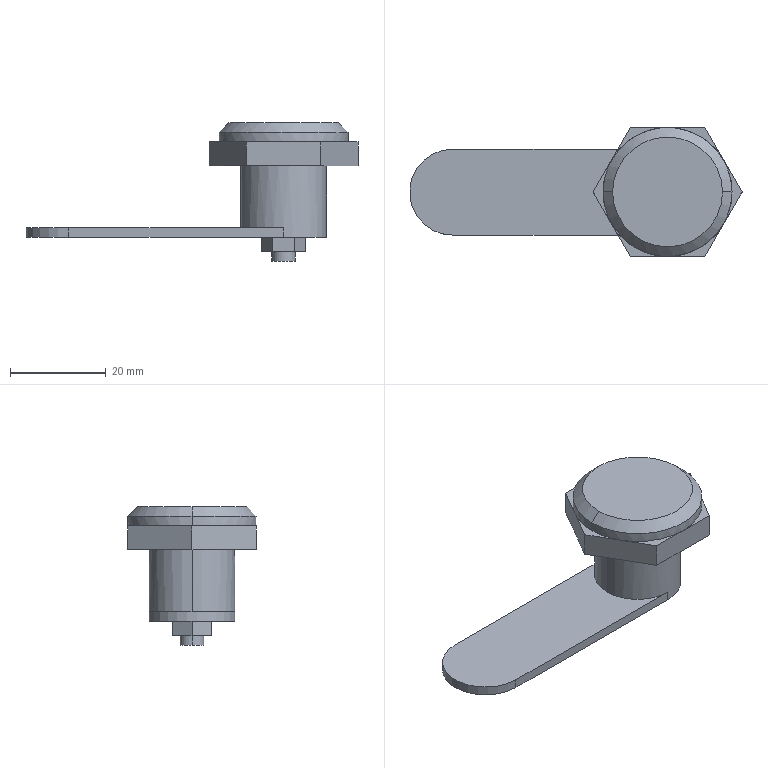Part | SolidWorks | features ICE 5, Chamfer 1, Extrusion 1 | 1 solid | 35 faces | box 69.588 x 27 x 29 mm | volume 10928 mm3 | plane 26 | cylinder 7 | cone 2 | commonest cylinder face diameters 18 x3 5 x2 27 x2
STEP:
#1=CARTESIAN_POINT('',(-2.5,0.,-25.));
#2=VERTEX_POINT('',#1);
#3=CARTESIAN_POINT('',(2.5,0.,-25.));
#4=VERTEX_POINT('',#3);
#5=CARTESIAN_POINT('',(0.,0.,-25.));
#6=DIRECTION('',(0.,0.,-1.));
#7=DIRECTION('',(-1.,0.,0.));
#8=AXIS2_PLACEMENT_3D('',#5,#6,#7);
#9=CIRCLE('',#8,2.5);
#10=EDGE_CURVE('',#2,#4,#9,.T.);
#11=ORIENTED_EDGE('',*,*,#10,.F.);
#12=CARTESIAN_POINT('',(-2.5,0.,-23.));
#13=VERTEX_POINT('',#12);
#14=CARTESIAN_POINT('',(-2.5,0.,-25.));
#15=DIRECTION('',(0.,0.,1.));
#16=VECTOR('',#15,1000.);
#17=LINE('',#14,#16);
#18=EDGE_CURVE('',#2,#13,#17,.T.);
#19=ORIENTED_EDGE('',*,*,#18,.T.);
#20=CARTESIAN_POINT('',(2.5,0.,-23.));
#21=VERTEX_POINT('',#20);
#22=CARTESIAN_POINT('',(0.,0.,-23.));
#23=DIRECTION('',(0.,0.,-1.));
#24=DIRECTION('',(-1.,0.,0.));
#25=AXIS2_PLACEMENT_3D('',#22,#23,#24);
#26=CIRCLE('',#25,2.5);
#27=EDGE_CURVE('',#13,#21,#26,.T.);
#28=ORIENTED_EDGE('',*,*,#27,.T.);
#29=CARTESIAN_POINT('',(2.5,0.,-25.));
#30=DIRECTION('',(0.,0.,1.));
#31=VECTOR('',#30,1000.);
#32=LINE('',#29,#31);
#33=EDGE_CURVE('',#4,#21,#32,.T.);
#34=ORIENTED_EDGE('',*,*,#33,.F.);
#35=EDGE_LOOP('',(#11,#19,#28,#34));
#36=FACE_OUTER_BOUND('',#35,.T.);
#37=CARTESIAN_POINT('',(0.,0.,-25.));
#38=DIRECTION('',(0.,0.,1.));
#39=DIRECTION('',(1.,0.,0.));
#40=AXIS2_PLACEMENT_3D('',#37,#38,#39);
#41=CYLINDRICAL_SURFACE('',#40,2.5);
#42=ADVANCED_FACE('',(#36),#41,.T.);
#43=CARTESIAN_POINT('',(-9.,0.,-18.));
#44=VERTEX_POINT('',#43);
#45=CARTESIAN_POINT('',(0.,9.,-18.));
#46=VERTEX_POINT('',#45);
#47=CARTESIAN_POINT('',(0.,0.,-18.));
#48=DIRECTION('',(0.,0.,-1.));
#49=DIRECTION('',(-1.,0.,0.));
#50=AXIS2_PLACEMENT_3D('',#47,#48,#49);
#51=CIRCLE('',#50,9.);
#52=EDGE_CURVE('',#44,#46,#51,.T.);
#53=ORIENTED_EDGE('',*,*,#52,.F.);
#54=CARTESIAN_POINT('',(-9.,0.,-5.));
#55=VERTEX_POINT('',#54);
#56=CARTESIAN_POINT('',(-9.,0.,-18.));
#57=DIRECTION('',(0.,0.,1.));
#58=VECTOR('',#57,1000.);
#59=LINE('',#56,#58);
#60=EDGE_CURVE('',#44,#55,#59,.T.);
#61=ORIENTED_EDGE('',*,*,#60,.T.);
#62=CARTESIAN_POINT('',(9.,0.,-5.));
#63=VERTEX_POINT('',#62);
#64=CARTESIAN_POINT('',(0.,0.,-5.));
#65=DIRECTION('',(0.,0.,-1.));
#66=DIRECTION('',(-1.,0.,0.));
#67=AXIS2_PLACEMENT_3D('',#64,#65,#66);
#68=CIRCLE('',#67,9.);
#69=EDGE_CURVE('',#55,#63,#68,.T.);
#70=ORIENTED_EDGE('',*,*,#69,.T.);
#71=CARTESIAN_POINT('',(9.,0.,-20.));
#72=VERTEX_POINT('',#71);
#73=CARTESIAN_POINT('',(9.,0.,-18.));
#74=DIRECTION('',(0.,0.,1.));
#75=VECTOR('',#74,1000.);
#76=LINE('',#73,#75);
#77=EDGE_CURVE('',#72,#63,#76,.T.);
#78=ORIENTED_EDGE('',*,*,#77,.F.);
#79=CARTESIAN_POINT('',(0.,9.,-20.));
#80=VERTEX_POINT('',#79);
#81=CARTESIAN_POINT('',(0.,0.,-20.));
#82=DIRECTION('',(0.,0.,-1.));
#83=DIRECTION('',(-1.,0.,0.));
#84=AXIS2_PLACEMENT_3D('',#81,#82,#83);
#85=CIRCLE('',#84,9.);
#86=EDGE_CURVE('',#80,#72,#85,.T.);
#87=ORIENTED_EDGE('',*,*,#86,.F.);
#88=CARTESIAN_POINT('',(0.,9.,-20.));
#89=DIRECTION('',(0.,0.,1.));
#90=VECTOR('',#89,1000.);
#91=LINE('',#88,#90);
#92=EDGE_CURVE('',#80,#46,#91,.T.);
#93=ORIENTED_EDGE('',*,*,#92,.T.);
#94=EDGE_LOOP('',(#53,#61,#70,#78,#87,#93));
#95=FACE_OUTER_BOUND('',#94,.T.);
#96=CARTESIAN_POINT('',(0.,0.,-18.));
#97=DIRECTION('',(0.,0.,1.));
#98=DIRECTION('',(1.,0.,0.));
#99=AXIS2_PLACEMENT_3D('',#96,#97,#98);
#100=CYLINDRICAL_SURFACE('',#99,9.);
#101=ADVANCED_FACE('',(#95),#100,.T.);
#102=CARTESIAN_POINT('',(11.5,0.,4.));
#103=VERTEX_POINT('',#102);
#104=CARTESIAN_POINT('',(-11.5,0.,4.));
#105=VERTEX_POINT('',#104);
#106=CARTESIAN_POINT('',(0.,0.,4.));
#107=DIRECTION('',(0.,0.,1.));
#108=DIRECTION('',(1.,0.,0.));
#109=AXIS2_PLACEMENT_3D('',#106,#107,#108);
#110=CIRCLE('',#109,11.5);
#111=EDGE_CURVE('',#103,#105,#110,.T.);
#112=ORIENTED_EDGE('',*,*,#111,.F.);
#113=CARTESIAN_POINT('',(13.5,0.,2.));
#114=VERTEX_POINT('',#113);
#115=CARTESIAN_POINT('',(11.5,0.,4.));
#116=DIRECTION('',(0.7071,0.,-0.7071));
#117=VECTOR('',#116,1000.);
#118=LINE('',#115,#117);
#119=EDGE_CURVE('',#103,#114,#118,.T.);
#120=ORIENTED_EDGE('',*,*,#119,.T.);
#121=CARTESIAN_POINT('',(-13.5,0.,2.));
#122=VERTEX_POINT('',#121);
#123=CARTESIAN_POINT('',(0.,0.,2.));
#124=DIRECTION('',(0.,0.,-1.));
#125=DIRECTION('',(1.,0.,0.));
#126=AXIS2_PLACEMENT_3D('',#123,#124,#125);
#127=CIRCLE('',#126,13.5);
#128=EDGE_CURVE('',#122,#114,#127,.T.);
#129=ORIENTED_EDGE('',*,*,#128,.F.);
#130=CARTESIAN_POINT('',(-11.5,0.,4.));
#131=DIRECTION('',(-0.7071,0.,-0.7071));
#132=VECTOR('',#131,1000.);
#133=LINE('',#130,#132);
#134=EDGE_CURVE('',#105,#122,#133,.T.);
#135=ORIENTED_EDGE('',*,*,#134,.F.);
#136=EDGE_LOOP('',(#112,#120,#129,#135));
#137=FACE_OUTER_BOUND('',#136,.T.);
#138=CARTESIAN_POINT('',(0.,0.,4.));
#139=DIRECTION('',(0.,0.,-1.));
#140=DIRECTION('',(-1.,0.,0.));
#141=AXIS2_PLACEMENT_3D('',#138,#139,#140);
#142=CONICAL_SURFACE('',#141,11.5,0.7854);
#143=ADVANCED_FACE('',(#137),#142,.T.);
#144=ORIENTED_EDGE('',*,*,#128,.T.);
#145=CARTESIAN_POINT('',(13.5,0.,0.));
#146=VERTEX_POINT('',#145);
#147=CARTESIAN_POINT('',(13.5,0.,4.));
#148=DIRECTION('',(0.,0.,-1.));
#149=VECTOR('',#148,1000.);
#150=LINE('',#147,#149);
#151=EDGE_CURVE('',#114,#146,#150,.T.);
#152=ORIENTED_EDGE('',*,*,#151,.T.);
#153=CARTESIAN_POINT('',(11.691,6.75,0.));
#154=VERTEX_POINT('',#153);
#155=CARTESIAN_POINT('',(0.,0.,0.));
#156=DIRECTION('',(0.,0.,1.));
#157=DIRECTION('',(1.,0.,0.));
#158=AXIS2_PLACEMENT_3D('',#155,#156,#157);
#159=CIRCLE('',#158,13.5);
#160=EDGE_CURVE('',#146,#154,#159,.T.);
#161=ORIENTED_EDGE('',*,*,#160,.T.);
#162=CARTESIAN_POINT('',(0.,13.5,0.));
#163=VERTEX_POINT('',#162);
#164=CARTESIAN_POINT('',(0.,0.,0.));
#165=DIRECTION('',(0.,0.,1.));
#166=DIRECTION('',(1.,0.,0.));
#167=AXIS2_PLACEMENT_3D('',#164,#165,#166);
#168=CIRCLE('',#167,13.5);
#169=EDGE_CURVE('',#154,#163,#168,.T.);
#170=ORIENTED_EDGE('',*,*,#169,.T.);
#171=CARTESIAN_POINT('',(-11.691,6.75,0.));
#172=VERTEX_POINT('',#171);
#173=CARTESIAN_POINT('',(0.,0.,0.));
#174=DIRECTION('',(0.,0.,1.));
#175=DIRECTION('',(1.,0.,0.));
#176=AXIS2_PLACEMENT_3D('',#173,#174,#175);
#177=CIRCLE('',#176,13.5);
#178=EDGE_CURVE('',#163,#172,#177,.T.);
#179=ORIENTED_EDGE('',*,*,#178,.T.);
#180=CARTESIAN_POINT('',(-13.5,0.,0.));
#181=VERTEX_POINT('',#180);
#182=CARTESIAN_POINT('',(0.,0.,0.));
#183=DIRECTION('',(0.,0.,1.));
#184=DIRECTION('',(1.,0.,0.));
#185=AXIS2_PLACEMENT_3D('',#182,#183,#184);
#186=CIRCLE('',#185,13.5);
#187=EDGE_CURVE('',#172,#181,#186,.T.);
#188=ORIENTED_EDGE('',*,*,#187,.T.);
#189=CARTESIAN_POINT('',(-13.5,0.,4.));
#190=DIRECTION('',(0.,0.,-1.));
#191=VECTOR('',#190,1000.);
#192=LINE('',#189,#191);
#193=EDGE_CURVE('',#122,#181,#192,.T.);
#194=ORIENTED_EDGE('',*,*,#193,.F.);
#195=EDGE_LOOP('',(#144,#152,#161,#170,#179,#188,#194));
#196=FACE_OUTER_BOUND('',#195,.T.);
#197=CARTESIAN_POINT('',(0.,0.,4.));
#198=DIRECTION('',(0.,0.,-1.));
#199=DIRECTION('',(-1.,0.,0.));
#200=AXIS2_PLACEMENT_3D('',#197,#198,#199);
#201=CYLINDRICAL_SURFACE('',#200,13.5);
#202=ADVANCED_FACE('',(#196),#201,.T.);
#203=ORIENTED_EDGE('',*,*,#86,.T.);
#204=CARTESIAN_POINT('',(0.,-9.,-20.));
#205=VERTEX_POINT('',#204);
#206=CARTESIAN_POINT('',(0.,0.,-20.));
#207=DIRECTION('',(0.,0.,-1.));
#208=DIRECTION('',(-1.,0.,0.));
#209=AXIS2_PLACEMENT_3D('',#206,#207,#208);
#210=CIRCLE('',#209,9.);
#211=EDGE_CURVE('',#72,#205,#210,.T.);
#212=ORIENTED_EDGE('',*,*,#211,.T.);
#213=CARTESIAN_POINT('',(-45.,-9.,-20.));
#214=VERTEX_POINT('',#213);
#215=CARTESIAN_POINT('',(0.,-9.,-20.));
#216=DIRECTION('',(-1.,0.,0.));
#217=VECTOR('',#216,1000.);
#218=LINE('',#215,#217);
#219=EDGE_CURVE('',#205,#214,#218,.T.);
#220=ORIENTED_EDGE('',*,*,#219,.T.);
#221=CARTESIAN_POINT('',(-45.,9.,-20.));
#222=VERTEX_POINT('',#221);
#223=CARTESIAN_POINT('',(-45.,0.,-20.));
#224=DIRECTION('',(0.,0.,-1.));
#225=DIRECTION('',(-1.,0.,0.));
#226=AXIS2_PLACEMENT_3D('',#223,#224,#225);
#227=CIRCLE('',#226,9.);
#228=EDGE_CURVE('',#214,#222,#227,.T.);
#229=ORIENTED_EDGE('',*,*,#228,.T.);
#230=CARTESIAN_POINT('',(0.,9.,-20.));
#231=DIRECTION('',(1.,0.,0.));
#232=VECTOR('',#231,1000.);
#233=LINE('',#230,#232);
#234=EDGE_CURVE('',#222,#80,#233,.T.);
#235=ORIENTED_EDGE('',*,*,#234,.T.);
#236=EDGE_LOOP('',(#203,#212,#220,#229,#235));
#237=FACE_OUTER_BOUND('',#236,.T.);
#238=CARTESIAN_POINT('',(2.309,-4.,-20.));
#239=VERTEX_POINT('',#238);
#240=CARTESIAN_POINT('',(-2.309,-4.,-20.));
#241=VERTEX_POINT('',#240);
#242=CARTESIAN_POINT('',(2.309,-4.,-20.));
#243=DIRECTION('',(-1.,0.,0.));
#244=VECTOR('',#243,1000.);
#245=LINE('',#242,#244);
#246=EDGE_CURVE('',#239,#241,#245,.T.);
#247=ORIENTED_EDGE('',*,*,#246,.F.);
#248=CARTESIAN_POINT('',(4.619,0.,-20.));
#249=VERTEX_POINT('',#248);
#250=CARTESIAN_POINT('',(4.619,0.,-20.));
#251=DIRECTION('',(-0.5,-0.866,0.));
#252=VECTOR('',#251,1000.);
#253=LINE('',#250,#252);
#254=EDGE_CURVE('',#249,#239,#253,.T.);
#255=ORIENTED_EDGE('',*,*,#254,.F.);
#256=CARTESIAN_POINT('',(2.309,4.,-20.));
#257=VERTEX_POINT('',#256);
#258=CARTESIAN_POINT('',(2.309,4.,-20.));
#259=DIRECTION('',(0.5,-0.866,0.));
#260=VECTOR('',#259,1000.);
#261=LINE('',#258,#260);
#262=EDGE_CURVE('',#257,#249,#261,.T.);
#263=ORIENTED_EDGE('',*,*,#262,.F.);
#264=CARTESIAN_POINT('',(-2.309,4.,-20.));
#265=VERTEX_POINT('',#264);
#266=CARTESIAN_POINT('',(-2.309,4.,-20.));
#267=DIRECTION('',(1.,0.,0.));
#268=VECTOR('',#267,1000.);
#269=LINE('',#266,#268);
#270=EDGE_CURVE('',#265,#257,#269,.T.);
#271=ORIENTED_EDGE('',*,*,#270,.F.);
#272=CARTESIAN_POINT('',(-4.619,0.,-20.));
#273=VERTEX_POINT('',#272);
#274=CARTESIAN_POINT('',(-4.619,0.,-20.));
#275=DIRECTION('',(0.5,0.866,0.));
#276=VECTOR('',#275,1000.);
#277=LINE('',#274,#276);
#278=EDGE_CURVE('',#273,#265,#277,.T.);
#279=ORIENTED_EDGE('',*,*,#278,.F.);
#280=CARTESIAN_POINT('',(-2.309,-4.,-20.));
#281=DIRECTION('',(-0.5,0.866,0.));
#282=VECTOR('',#281,1000.);
#283=LINE('',#280,#282);
#284=EDGE_CURVE('',#241,#273,#283,.T.);
#285=ORIENTED_EDGE('',*,*,#284,.F.);
#286=EDGE_LOOP('',(#247,#255,#263,#271,#279,#285));
#287=FACE_BOUND('',#286,.T.);
#288=CARTESIAN_POINT('',(0.,0.,-20.));
#289=DIRECTION('',(0.,0.,-1.));
#290=DIRECTION('',(-1.,0.,0.));
#291=AXIS2_PLACEMENT_3D('',#288,#289,#290);
#292=PLANE('',#291);
#293=ADVANCED_FACE('',(#237,#287),#292,.T.);
#294=CARTESIAN_POINT('',(7.794,13.5,-5.));
#295=VERTEX_POINT('',#294);
#296=CARTESIAN_POINT('',(15.588,0.,-5.));
#297=VERTEX_POINT('',#296);
#298=CARTESIAN_POINT('',(7.794,13.5,-5.));
#299=DIRECTION('',(0.5,-0.866,0.));
#300=VECTOR('',#299,1000.);
#301=LINE('',#298,#300);
#302=EDGE_CURVE('',#295,#297,#301,.T.);
#303=ORIENTED_EDGE('',*,*,#302,.T.);
#304=CARTESIAN_POINT('',(7.794,-13.5,-5.));
#305=VERTEX_POINT('',#304);
#306=CARTESIAN_POINT('',(15.588,0.,-5.));
#307=DIRECTION('',(-0.5,-0.866,0.));
#308=VECTOR('',#307,1000.);
#309=LINE('',#306,#308);
#310=EDGE_CURVE('',#297,#305,#309,.T.);
#311=ORIENTED_EDGE('',*,*,#310,.T.);
#312=CARTESIAN_POINT('',(-7.794,-13.5,-5.));
#313=VERTEX_POINT('',#312);
#314=CARTESIAN_POINT('',(7.794,-13.5,-5.));
#315=DIRECTION('',(-1.,0.,0.));
#316=VECTOR('',#315,1000.);
#317=LINE('',#314,#316);
#318=EDGE_CURVE('',#305,#313,#317,.T.);
#319=ORIENTED_EDGE('',*,*,#318,.T.);
#320=CARTESIAN_POINT('',(-15.588,0.,-5.));
#321=VERTEX_POINT('',#320);
#322=CARTESIAN_POINT('',(-7.794,-13.5,-5.));
#323=DIRECTION('',(-0.5,0.866,0.));
#324=VECTOR('',#323,1000.);
#325=LINE('',#322,#324);
#326=EDGE_CURVE('',#313,#321,#325,.T.);
#327=ORIENTED_EDGE('',*,*,#326,.T.);
#328=CARTESIAN_POINT('',(-7.794,13.5,-5.));
#329=VERTEX_POINT('',#328);
#330=CARTESIAN_POINT('',(-15.588,0.,-5.));
#331=DIRECTION('',(0.5,0.866,0.));
#332=VECTOR('',#331,1000.);
#333=LINE('',#330,#332);
#334=EDGE_CURVE('',#321,#329,#333,.T.);
#335=ORIENTED_EDGE('',*,*,#334,.T.);
#336=CARTESIAN_POINT('',(-7.794,13.5,-5.));
#337=DIRECTION('',(1.,0.,0.));
#338=VECTOR('',#337,1000.);
#339=LINE('',#336,#338);
#340=EDGE_CURVE('',#329,#295,#339,.T.);
#341=ORIENTED_EDGE('',*,*,#340,.T.);
#342=EDGE_LOOP('',(#303,#311,#319,#327,#335,#341));
#343=FACE_OUTER_BOUND('',#342,.T.);
#344=CARTESIAN_POINT('',(0.,0.,-5.));
#345=DIRECTION('',(0.,0.,-1.));
#346=DIRECTION('',(-1.,0.,0.));
#347=AXIS2_PLACEMENT_3D('',#344,#345,#346);
#348=CIRCLE('',#347,9.);
#349=EDGE_CURVE('',#63,#55,#348,.T.);
#350=ORIENTED_EDGE('',*,*,#349,.F.);
#351=ORIENTED_EDGE('',*,*,#69,.F.);
#352=EDGE_LOOP('',(#350,#351));
#353=FACE_BOUND('',#352,.T.);
#354=CARTESIAN_POINT('',(15.588,0.,-5.));
#355=DIRECTION('',(0.,0.,-1.));
#356=DIRECTION('',(-1.,0.,0.));
#357=AXIS2_PLACEMENT_3D('',#354,#355,#356);
#358=PLANE('',#357);
#359=ADVANCED_FACE('',(#343,#353),#358,.T.);
#360=ORIENTED_EDGE('',*,*,#151,.F.);
#361=CARTESIAN_POINT('',(0.,0.,2.));
#362=DIRECTION('',(0.,0.,-1.));
#363=DIRECTION('',(1.,0.,0.));
#364=AXIS2_PLACEMENT_3D('',#361,#362,#363);
#365=CIRCLE('',#364,13.5);
#366=EDGE_CURVE('',#114,#122,#365,.T.);
#367=ORIENTED_EDGE('',*,*,#366,.T.);
#368=ORIENTED_EDGE('',*,*,#193,.T.);
#369=CARTESIAN_POINT('',(-11.691,-6.75,0.));
#370=VERTEX_POINT('',#369);
#371=CARTESIAN_POINT('',(0.,0.,0.));
#372=DIRECTION('',(0.,0.,1.));
#373=DIRECTION('',(1.,0.,0.));
#374=AXIS2_PLACEMENT_3D('',#371,#372,#373);
#375=CIRCLE('',#374,13.5);
#376=EDGE_CURVE('',#181,#370,#375,.T.);
#377=ORIENTED_EDGE('',*,*,#376,.T.);
#378=CARTESIAN_POINT('',(0.,-13.5,0.));
#379=VERTEX_POINT('',#378);
#380=CARTESIAN_POINT('',(0.,0.,0.));
#381=DIRECTION('',(0.,0.,1.));
#382=DIRECTION('',(1.,0.,0.));
#383=AXIS2_PLACEMENT_3D('',#380,#381,#382);
#384=CIRCLE('',#383,13.5);
#385=EDGE_CURVE('',#370,#379,#384,.T.);
#386=ORIENTED_EDGE('',*,*,#385,.T.);
#387=CARTESIAN_POINT('',(11.691,-6.75,0.));
#388=VERTEX_POINT('',#387);
#389=CARTESIAN_POINT('',(0.,0.,0.));
#390=DIRECTION('',(0.,0.,1.));
#391=DIRECTION('',(1.,0.,0.));
#392=AXIS2_PLACEMENT_3D('',#389,#390,#391);
#393=CIRCLE('',#392,13.5);
#394=EDGE_CURVE('',#379,#388,#393,.T.);
#395=ORIENTED_EDGE('',*,*,#394,.T.);
#396=CARTESIAN_POINT('',(0.,0.,0.));
#397=DIRECTION('',(0.,0.,1.));
#398=DIRECTION('',(1.,0.,0.));
#399=AXIS2_PLACEMENT_3D('',#396,#397,#398);
#400=CIRCLE('',#399,13.5);
#401=EDGE_CURVE('',#388,#146,#400,.T.);
#402=ORIENTED_EDGE('',*,*,#401,.T.);
#403=EDGE_LOOP('',(#360,#367,#368,#377,#386,#395,#402));
#404=FACE_OUTER_BOUND('',#403,.T.);
#405=CARTESIAN_POINT('',(0.,0.,4.));
#406=DIRECTION('',(0.,0.,-1.));
#407=DIRECTION('',(-1.,0.,0.));
#408=AXIS2_PLACEMENT_3D('',#405,#406,#407);
#409=CYLINDRICAL_SURFACE('',#408,13.5);
#410=ADVANCED_FACE('',(#404),#409,.T.);
#411=CARTESIAN_POINT('',(0.,0.,4.));
#412=DIRECTION('',(0.,0.,1.));
#413=DIRECTION('',(1.,0.,0.));
#414=AXIS2_PLACEMENT_3D('',#411,#412,#413);
#415=CIRCLE('',#414,11.5);
#416=EDGE_CURVE('',#105,#103,#415,.T.);
#417=ORIENTED_EDGE('',*,*,#416,.T.);
#418=ORIENTED_EDGE('',*,*,#111,.T.);
#419=EDGE_LOOP('',(#417,#418));
#420=FACE_OUTER_BOUND('',#419,.T.);
#421=CARTESIAN_POINT('',(0.,0.,4.));
#422=DIRECTION('',(0.,0.,1.));
#423=DIRECTION('',(1.,0.,0.));
#424=AXIS2_PLACEMENT_3D('',#421,#422,#423);
#425=PLANE('',#424);
#426=ADVANCED_FACE('',(#420),#425,.T.);
#427=ORIENTED_EDGE('',*,*,#119,.F.);
#428=ORIENTED_EDGE('',*,*,#416,.F.);
#429=ORIENTED_EDGE('',*,*,#134,.T.);
#430=ORIENTED_EDGE('',*,*,#366,.F.);
#431=EDGE_LOOP('',(#427,#428,#429,#430));
#432=FACE_OUTER_BOUND('',#431,.T.);
#433=CARTESIAN_POINT('',(0.,0.,4.));
#434=DIRECTION('',(0.,0.,-1.));
#435=DIRECTION('',(-1.,0.,0.));
#436=AXIS2_PLACEMENT_3D('',#433,#434,#435);
#437=CONICAL_SURFACE('',#436,11.5,0.7854);
#438=ADVANCED_FACE('',(#432),#437,.T.);
#439=ORIENTED_EDGE('',*,*,#169,.F.);
#440=CARTESIAN_POINT('',(7.794,13.5,0.));
#441=VERTEX_POINT('',#440);
#442=CARTESIAN_POINT('',(7.794,13.5,0.));
#443=DIRECTION('',(0.5,-0.866,0.));
#444=VECTOR('',#443,1000.);
#445=LINE('',#442,#444);
#446=EDGE_CURVE('',#441,#154,#445,.T.);
#447=ORIENTED_EDGE('',*,*,#446,.F.);
#448=CARTESIAN_POINT('',(-7.794,13.5,0.));
#449=DIRECTION('',(1.,0.,0.));
#450=VECTOR('',#449,1000.);
#451=LINE('',#448,#450);
#452=EDGE_CURVE('',#163,#441,#451,.T.);
#453=ORIENTED_EDGE('',*,*,#452,.F.);
#454=EDGE_LOOP('',(#439,#447,#453));
#455=FACE_OUTER_BOUND('',#454,.T.);
#456=CARTESIAN_POINT('',(15.588,0.,0.));
#457=DIRECTION('',(0.,0.,-1.));
#458=DIRECTION('',(-1.,0.,0.));
#459=AXIS2_PLACEMENT_3D('',#456,#457,#458);
#460=PLANE('',#459);
#461=ADVANCED_FACE('',(#455),#460,.F.);
#462=ORIENTED_EDGE('',*,*,#178,.F.);
#463=CARTESIAN_POINT('',(-7.794,13.5,0.));
#464=VERTEX_POINT('',#463);
#465=CARTESIAN_POINT('',(-7.794,13.5,0.));
#466=DIRECTION('',(1.,0.,0.));
#467=VECTOR('',#466,1000.);
#468=LINE('',#465,#467);
#469=EDGE_CURVE('',#464,#163,#468,.T.);
#470=ORIENTED_EDGE('',*,*,#469,.F.);
#471=CARTESIAN_POINT('',(-15.588,0.,0.));
#472=DIRECTION('',(0.5,0.866,0.));
#473=VECTOR('',#472,1000.);
#474=LINE('',#471,#473);
#475=EDGE_CURVE('',#172,#464,#474,.T.);
#476=ORIENTED_EDGE('',*,*,#475,.F.);
#477=EDGE_LOOP('',(#462,#470,#476));
#478=FACE_OUTER_BOUND('',#477,.T.);
#479=CARTESIAN_POINT('',(15.588,0.,0.));
#480=DIRECTION('',(0.,0.,-1.));
#481=DIRECTION('',(-1.,0.,0.));
#482=AXIS2_PLACEMENT_3D('',#479,#480,#481);
#483=PLANE('',#482);
#484=ADVANCED_FACE('',(#478),#483,.F.);
#485=ORIENTED_EDGE('',*,*,#187,.F.);
#486=CARTESIAN_POINT('',(-15.588,0.,0.));
#487=VERTEX_POINT('',#486);
#488=CARTESIAN_POINT('',(-15.588,0.,0.));
#489=DIRECTION('',(0.5,0.866,0.));
#490=VECTOR('',#489,1000.);
#491=LINE('',#488,#490);
#492=EDGE_CURVE('',#487,#172,#491,.T.);
#493=ORIENTED_EDGE('',*,*,#492,.F.);
#494=CARTESIAN_POINT('',(-7.794,-13.5,0.));
#495=DIRECTION('',(-0.5,0.866,0.));
#496=VECTOR('',#495,1000.);
#497=LINE('',#494,#496);
#498=EDGE_CURVE('',#370,#487,#497,.T.);
#499=ORIENTED_EDGE('',*,*,#498,.F.);
#500=ORIENTED_EDGE('',*,*,#376,.F.);
#501=EDGE_LOOP('',(#485,#493,#499,#500));
#502=FACE_OUTER_BOUND('',#501,.T.);
#503=CARTESIAN_POINT('',(15.588,0.,0.));
#504=DIRECTION('',(0.,0.,-1.));
#505=DIRECTION('',(-1.,0.,0.));
#506=AXIS2_PLACEMENT_3D('',#503,#504,#505);
#507=PLANE('',#506);
#508=ADVANCED_FACE('',(#502),#507,.F.);
#509=ORIENTED_EDGE('',*,*,#385,.F.);
#510=CARTESIAN_POINT('',(-7.794,-13.5,0.));
#511=VERTEX_POINT('',#510);
#512=CARTESIAN_POINT('',(-7.794,-13.5,0.));
#513=DIRECTION('',(-0.5,0.866,0.));
#514=VECTOR('',#513,1000.);
#515=LINE('',#512,#514);
#516=EDGE_CURVE('',#511,#370,#515,.T.);
#517=ORIENTED_EDGE('',*,*,#516,.F.);
#518=CARTESIAN_POINT('',(7.794,-13.5,0.));
#519=DIRECTION('',(-1.,0.,0.));
#520=VECTOR('',#519,1000.);
#521=LINE('',#518,#520);
#522=EDGE_CURVE('',#379,#511,#521,.T.);
#523=ORIENTED_EDGE('',*,*,#522,.F.);
#524=EDGE_LOOP('',(#509,#517,#523));
#525=FACE_OUTER_BOUND('',#524,.T.);
#526=CARTESIAN_POINT('',(15.588,0.,0.));
#527=DIRECTION('',(0.,0.,-1.));
#528=DIRECTION('',(-1.,0.,0.));
#529=AXIS2_PLACEMENT_3D('',#526,#527,#528);
#530=PLANE('',#529);
#531=ADVANCED_FACE('',(#525),#530,.F.);
#532=ORIENTED_EDGE('',*,*,#394,.F.);
#533=CARTESIAN_POINT('',(7.794,-13.5,0.));
#534=VERTEX_POINT('',#533);
#535=CARTESIAN_POINT('',(7.794,-13.5,0.));
#536=DIRECTION('',(-1.,0.,0.));
#537=VECTOR('',#536,1000.);
#538=LINE('',#535,#537);
#539=EDGE_CURVE('',#534,#379,#538,.T.);
#540=ORIENTED_EDGE('',*,*,#539,.F.);
#541=CARTESIAN_POINT('',(15.588,0.,0.));
#542=DIRECTION('',(-0.5,-0.866,0.));
#543=VECTOR('',#542,1000.);
#544=LINE('',#541,#543);
#545=EDGE_CURVE('',#388,#534,#544,.T.);
#546=ORIENTED_EDGE('',*,*,#545,.F.);
#547=EDGE_LOOP('',(#532,#540,#546));
#548=FACE_OUTER_BOUND('',#547,.T.);
#549=CARTESIAN_POINT('',(15.588,0.,0.));
#550=DIRECTION('',(0.,0.,-1.));
#551=DIRECTION('',(-1.,0.,0.));
#552=AXIS2_PLACEMENT_3D('',#549,#550,#551);
#553=PLANE('',#552);
#554=ADVANCED_FACE('',(#548),#553,.F.);
#555=ORIENTED_EDGE('',*,*,#446,.T.);
#556=CARTESIAN_POINT('',(15.588,0.,0.));
#557=VERTEX_POINT('',#556);
#558=CARTESIAN_POINT('',(7.794,13.5,0.));
#559=DIRECTION('',(0.5,-0.866,0.));
#560=VECTOR('',#559,1000.);
#561=LINE('',#558,#560);
#562=EDGE_CURVE('',#154,#557,#561,.T.);
#563=ORIENTED_EDGE('',*,*,#562,.T.);
#564=CARTESIAN_POINT('',(15.588,0.,-5.));
#565=DIRECTION('',(0.,0.,1.));
#566=VECTOR('',#565,1000.);
#567=LINE('',#564,#566);
#568=EDGE_CURVE('',#297,#557,#567,.T.);
#569=ORIENTED_EDGE('',*,*,#568,.F.);
#570=ORIENTED_EDGE('',*,*,#302,.F.);
#571=CARTESIAN_POINT('',(7.794,13.5,-5.));
#572=DIRECTION('',(0.,0.,1.));
#573=VECTOR('',#572,1000.);
#574=LINE('',#571,#573);
#575=EDGE_CURVE('',#295,#441,#574,.T.);
#576=ORIENTED_EDGE('',*,*,#575,.T.);
#577=EDGE_LOOP('',(#555,#563,#569,#570,#576));
#578=FACE_OUTER_BOUND('',#577,.T.);
#579=CARTESIAN_POINT('',(7.794,13.5,-5.));
#580=DIRECTION('',(-0.866,-0.5,0.));
#581=DIRECTION('',(0.5,-0.866,0.));
#582=AXIS2_PLACEMENT_3D('',#579,#580,#581);
#583=PLANE('',#582);
#584=ADVANCED_FACE('',(#578),#583,.F.);
#585=CARTESIAN_POINT('',(15.588,0.,0.));
#586=DIRECTION('',(-0.5,-0.866,0.));
#587=VECTOR('',#586,1000.);
#588=LINE('',#585,#587);
#589=EDGE_CURVE('',#557,#388,#588,.T.);
#590=ORIENTED_EDGE('',*,*,#589,.T.);
#591=ORIENTED_EDGE('',*,*,#545,.T.);
#592=CARTESIAN_POINT('',(7.794,-13.5,-5.));
#593=DIRECTION('',(0.,0.,1.));
#594=VECTOR('',#593,1000.);
#595=LINE('',#592,#594);
#596=EDGE_CURVE('',#305,#534,#595,.T.);
#597=ORIENTED_EDGE('',*,*,#596,.F.);
#598=ORIENTED_EDGE('',*,*,#310,.F.);
#599=ORIENTED_EDGE('',*,*,#568,.T.);
#600=EDGE_LOOP('',(#590,#591,#597,#598,#599));
#601=FACE_OUTER_BOUND('',#600,.T.);
#602=CARTESIAN_POINT('',(15.588,0.,-5.));
#603=DIRECTION('',(-0.866,0.5,0.));
#604=DIRECTION('',(-0.5,-0.866,0.));
#605=AXIS2_PLACEMENT_3D('',#602,#603,#604);
#606=PLANE('',#605);
#607=ADVANCED_FACE('',(#601),#606,.F.);
#608=ORIENTED_EDGE('',*,*,#539,.T.);
#609=ORIENTED_EDGE('',*,*,#522,.T.);
#610=CARTESIAN_POINT('',(-7.794,-13.5,-5.));
#611=DIRECTION('',(0.,0.,1.));
#612=VECTOR('',#611,1000.);
#613=LINE('',#610,#612);
#614=EDGE_CURVE('',#313,#511,#613,.T.);
#615=ORIENTED_EDGE('',*,*,#614,.F.);
#616=ORIENTED_EDGE('',*,*,#318,.F.);
#617=ORIENTED_EDGE('',*,*,#596,.T.);
#618=EDGE_LOOP('',(#608,#609,#615,#616,#617));
#619=FACE_OUTER_BOUND('',#618,.T.);
#620=CARTESIAN_POINT('',(7.794,-13.5,-5.));
#621=DIRECTION('',(0.,1.,0.));
#622=DIRECTION('',(0.,0.,1.));
#623=AXIS2_PLACEMENT_3D('',#620,#621,#622);
#624=PLANE('',#623);
#625=ADVANCED_FACE('',(#619),#624,.F.);
#626=ORIENTED_EDGE('',*,*,#516,.T.);
#627=ORIENTED_EDGE('',*,*,#498,.T.);
#628=CARTESIAN_POINT('',(-15.588,0.,-5.));
#629=DIRECTION('',(0.,0.,1.));
#630=VECTOR('',#629,1000.);
#631=LINE('',#628,#630);
#632=EDGE_CURVE('',#321,#487,#631,.T.);
#633=ORIENTED_EDGE('',*,*,#632,.F.);
#634=ORIENTED_EDGE('',*,*,#326,.F.);
#635=ORIENTED_EDGE('',*,*,#614,.T.);
#636=EDGE_LOOP('',(#626,#627,#633,#634,#635));
#637=FACE_OUTER_BOUND('',#636,.T.);
#638=CARTESIAN_POINT('',(-7.794,-13.5,-5.));
#639=DIRECTION('',(0.866,0.5,0.));
#640=DIRECTION('',(-0.5,0.866,0.));
#641=AXIS2_PLACEMENT_3D('',#638,#639,#640);
#642=PLANE('',#641);
#643=ADVANCED_FACE('',(#637),#642,.F.);
#644=ORIENTED_EDGE('',*,*,#492,.T.);
#645=ORIENTED_EDGE('',*,*,#475,.T.);
#646=CARTESIAN_POINT('',(-7.794,13.5,-5.));
#647=DIRECTION('',(0.,0.,1.));
#648=VECTOR('',#647,1000.);
#649=LINE('',#646,#648);
#650=EDGE_CURVE('',#329,#464,#649,.T.);
#651=ORIENTED_EDGE('',*,*,#650,.F.);
#652=ORIENTED_EDGE('',*,*,#334,.F.);
#653=ORIENTED_EDGE('',*,*,#632,.T.);
#654=EDGE_LOOP('',(#644,#645,#651,#652,#653));
#655=FACE_OUTER_BOUND('',#654,.T.);
#656=CARTESIAN_POINT('',(-15.588,0.,-5.));
#657=DIRECTION('',(0.866,-0.5,0.));
#658=DIRECTION('',(0.5,0.866,0.));
#659=AXIS2_PLACEMENT_3D('',#656,#657,#658);
#660=PLANE('',#659);
#661=ADVANCED_FACE('',(#655),#660,.F.);
#662=ORIENTED_EDGE('',*,*,#469,.T.);
#663=ORIENTED_EDGE('',*,*,#452,.T.);
#664=ORIENTED_EDGE('',*,*,#575,.F.);
#665=ORIENTED_EDGE('',*,*,#340,.F.);
#666=ORIENTED_EDGE('',*,*,#650,.T.);
#667=EDGE_LOOP('',(#662,#663,#664,#665,#666));
#668=FACE_OUTER_BOUND('',#667,.T.);
#669=CARTESIAN_POINT('',(-7.794,13.5,-5.));
#670=DIRECTION('',(0.,-1.,0.));
#671=DIRECTION('',(1.,0.,0.));
#672=AXIS2_PLACEMENT_3D('',#669,#670,#671);
#673=PLANE('',#672);
#674=ADVANCED_FACE('',(#668),#673,.F.);
#675=ORIENTED_EDGE('',*,*,#401,.F.);
#676=ORIENTED_EDGE('',*,*,#589,.F.);
#677=ORIENTED_EDGE('',*,*,#562,.F.);
#678=ORIENTED_EDGE('',*,*,#160,.F.);
#679=EDGE_LOOP('',(#675,#676,#677,#678));
#680=FACE_OUTER_BOUND('',#679,.T.);
#681=CARTESIAN_POINT('',(15.588,0.,0.));
#682=DIRECTION('',(0.,0.,-1.));
#683=DIRECTION('',(-1.,0.,0.));
#684=AXIS2_PLACEMENT_3D('',#681,#682,#683);
#685=PLANE('',#684);
#686=ADVANCED_FACE('',(#680),#685,.F.);
#687=ORIENTED_EDGE('',*,*,#60,.F.);
#688=CARTESIAN_POINT('',(0.,-9.,-18.));
#689=VERTEX_POINT('',#688);
#690=CARTESIAN_POINT('',(0.,0.,-18.));
#691=DIRECTION('',(0.,0.,-1.));
#692=DIRECTION('',(-1.,0.,0.));
#693=AXIS2_PLACEMENT_3D('',#690,#691,#692);
#694=CIRCLE('',#693,9.);
#695=EDGE_CURVE('',#689,#44,#694,.T.);
#696=ORIENTED_EDGE('',*,*,#695,.F.);
#697=CARTESIAN_POINT('',(0.,-9.,-20.));
#698=DIRECTION('',(0.,0.,1.));
#699=VECTOR('',#698,1000.);
#700=LINE('',#697,#699);
#701=EDGE_CURVE('',#205,#689,#700,.T.);
#702=ORIENTED_EDGE('',*,*,#701,.F.);
#703=ORIENTED_EDGE('',*,*,#211,.F.);
#704=ORIENTED_EDGE('',*,*,#77,.T.);
#705=ORIENTED_EDGE('',*,*,#349,.T.);
#706=EDGE_LOOP('',(#687,#696,#702,#703,#704,#705));
#707=FACE_OUTER_BOUND('',#706,.T.);
#708=CARTESIAN_POINT('',(0.,0.,-18.));
#709=DIRECTION('',(0.,0.,1.));
#710=DIRECTION('',(1.,0.,0.));
#711=AXIS2_PLACEMENT_3D('',#708,#709,#710);
#712=CYLINDRICAL_SURFACE('',#711,9.);
#713=ADVANCED_FACE('',(#707),#712,.T.);
#714=CARTESIAN_POINT('',(-45.,-9.,-18.));
#715=VERTEX_POINT('',#714);
#716=CARTESIAN_POINT('',(0.,-9.,-18.));
#717=DIRECTION('',(-1.,0.,0.));
#718=VECTOR('',#717,1000.);
#719=LINE('',#716,#718);
#720=EDGE_CURVE('',#689,#715,#719,.T.);
#721=ORIENTED_EDGE('',*,*,#720,.F.);
#722=ORIENTED_EDGE('',*,*,#695,.T.);
#723=ORIENTED_EDGE('',*,*,#52,.T.);
#724=CARTESIAN_POINT('',(-45.,9.,-18.));
#725=VERTEX_POINT('',#724);
#726=CARTESIAN_POINT('',(0.,9.,-18.));
#727=DIRECTION('',(1.,0.,0.));
#728=VECTOR('',#727,1000.);
#729=LINE('',#726,#728);
#730=EDGE_CURVE('',#725,#46,#729,.T.);
#731=ORIENTED_EDGE('',*,*,#730,.F.);
#732=CARTESIAN_POINT('',(-45.,0.,-18.));
#733=DIRECTION('',(0.,0.,-1.));
#734=DIRECTION('',(-1.,0.,0.));
#735=AXIS2_PLACEMENT_3D('',#732,#733,#734);
#736=CIRCLE('',#735,9.);
#737=EDGE_CURVE('',#715,#725,#736,.T.);
#738=ORIENTED_EDGE('',*,*,#737,.F.);
#739=EDGE_LOOP('',(#721,#722,#723,#731,#738));
#740=FACE_OUTER_BOUND('',#739,.T.);
#741=CARTESIAN_POINT('',(0.,0.,-18.));
#742=DIRECTION('',(0.,0.,-1.));
#743=DIRECTION('',(-1.,0.,0.));
#744=AXIS2_PLACEMENT_3D('',#741,#742,#743);
#745=PLANE('',#744);
#746=ADVANCED_FACE('',(#740),#745,.F.);
#747=ORIENTED_EDGE('',*,*,#720,.T.);
#748=CARTESIAN_POINT('',(-45.,-9.,-20.));
#749=DIRECTION('',(0.,0.,1.));
#750=VECTOR('',#749,1000.);
#751=LINE('',#748,#750);
#752=EDGE_CURVE('',#214,#715,#751,.T.);
#753=ORIENTED_EDGE('',*,*,#752,.F.);
#754=ORIENTED_EDGE('',*,*,#219,.F.);
#755=ORIENTED_EDGE('',*,*,#701,.T.);
#756=EDGE_LOOP('',(#747,#753,#754,#755));
#757=FACE_OUTER_BOUND('',#756,.T.);
#758=CARTESIAN_POINT('',(0.,-9.,-20.));
#759=DIRECTION('',(0.,1.,0.));
#760=DIRECTION('',(-1.,0.,0.));
#761=AXIS2_PLACEMENT_3D('',#758,#759,#760);
#762=PLANE('',#761);
#763=ADVANCED_FACE('',(#757),#762,.F.);
#764=ORIENTED_EDGE('',*,*,#737,.T.);
#765=CARTESIAN_POINT('',(-45.,9.,-20.));
#766=DIRECTION('',(0.,0.,1.));
#767=VECTOR('',#766,1000.);
#768=LINE('',#765,#767);
#769=EDGE_CURVE('',#222,#725,#768,.T.);
#770=ORIENTED_EDGE('',*,*,#769,.F.);
#771=ORIENTED_EDGE('',*,*,#228,.F.);
#772=ORIENTED_EDGE('',*,*,#752,.T.);
#773=EDGE_LOOP('',(#764,#770,#771,#772));
#774=FACE_OUTER_BOUND('',#773,.T.);
#775=CARTESIAN_POINT('',(-45.,0.,-20.));
#776=DIRECTION('',(0.,0.,1.));
#777=DIRECTION('',(1.,0.,0.));
#778=AXIS2_PLACEMENT_3D('',#775,#776,#777);
#779=CYLINDRICAL_SURFACE('',#778,9.);
#780=ADVANCED_FACE('',(#774),#779,.T.);
#781=ORIENTED_EDGE('',*,*,#730,.T.);
#782=ORIENTED_EDGE('',*,*,#92,.F.);
#783=ORIENTED_EDGE('',*,*,#234,.F.);
#784=ORIENTED_EDGE('',*,*,#769,.T.);
#785=EDGE_LOOP('',(#781,#782,#783,#784));
#786=FACE_OUTER_BOUND('',#785,.T.);
#787=CARTESIAN_POINT('',(0.,9.,-20.));
#788=DIRECTION('',(0.,-1.,0.));
#789=DIRECTION('',(1.,0.,0.));
#790=AXIS2_PLACEMENT_3D('',#787,#788,#789);
#791=PLANE('',#790);
#792=ADVANCED_FACE('',(#786),#791,.F.);
#793=CARTESIAN_POINT('',(4.619,0.,-23.));
#794=VERTEX_POINT('',#793);
#795=CARTESIAN_POINT('',(2.309,-4.,-23.));
#796=VERTEX_POINT('',#795);
#797=CARTESIAN_POINT('',(4.619,0.,-23.));
#798=DIRECTION('',(-0.5,-0.866,0.));
#799=VECTOR('',#798,1000.);
#800=LINE('',#797,#799);
#801=EDGE_CURVE('',#794,#796,#800,.T.);
#802=ORIENTED_EDGE('',*,*,#801,.T.);
#803=CARTESIAN_POINT('',(-2.309,-4.,-23.));
#804=VERTEX_POINT('',#803);
#805=CARTESIAN_POINT('',(2.309,-4.,-23.));
#806=DIRECTION('',(-1.,0.,0.));
#807=VECTOR('',#806,1000.);
#808=LINE('',#805,#807);
#809=EDGE_CURVE('',#796,#804,#808,.T.);
#810=ORIENTED_EDGE('',*,*,#809,.T.);
#811=CARTESIAN_POINT('',(-4.619,0.,-23.));
#812=VERTEX_POINT('',#811);
#813=CARTESIAN_POINT('',(-2.309,-4.,-23.));
#814=DIRECTION('',(-0.5,0.866,0.));
#815=VECTOR('',#814,1000.);
#816=LINE('',#813,#815);
#817=EDGE_CURVE('',#804,#812,#816,.T.);
#818=ORIENTED_EDGE('',*,*,#817,.T.);
#819=CARTESIAN_POINT('',(-2.309,4.,-23.));
#820=VERTEX_POINT('',#819);
#821=CARTESIAN_POINT('',(-4.619,0.,-23.));
#822=DIRECTION('',(0.5,0.866,0.));
#823=VECTOR('',#822,1000.);
#824=LINE('',#821,#823);
#825=EDGE_CURVE('',#812,#820,#824,.T.);
#826=ORIENTED_EDGE('',*,*,#825,.T.);
#827=CARTESIAN_POINT('',(2.309,4.,-23.));
#828=VERTEX_POINT('',#827);
#829=CARTESIAN_POINT('',(-2.309,4.,-23.));
#830=DIRECTION('',(1.,0.,0.));
#831=VECTOR('',#830,1000.);
#832=LINE('',#829,#831);
#833=EDGE_CURVE('',#820,#828,#832,.T.);
#834=ORIENTED_EDGE('',*,*,#833,.T.);
#835=CARTESIAN_POINT('',(2.309,4.,-23.));
#836=DIRECTION('',(0.5,-0.866,0.));
#837=VECTOR('',#836,1000.);
#838=LINE('',#835,#837);
#839=EDGE_CURVE('',#828,#794,#838,.T.);
#840=ORIENTED_EDGE('',*,*,#839,.T.);
#841=EDGE_LOOP('',(#802,#810,#818,#826,#834,#840));
#842=FACE_OUTER_BOUND('',#841,.T.);
#843=CARTESIAN_POINT('',(0.,0.,-23.));
#844=DIRECTION('',(0.,0.,-1.));
#845=DIRECTION('',(-1.,0.,0.));
#846=AXIS2_PLACEMENT_3D('',#843,#844,#845);
#847=CIRCLE('',#846,2.5);
#848=EDGE_CURVE('',#21,#13,#847,.T.);
#849=ORIENTED_EDGE('',*,*,#848,.F.);
#850=ORIENTED_EDGE('',*,*,#27,.F.);
#851=EDGE_LOOP('',(#849,#850));
#852=FACE_BOUND('',#851,.T.);
#853=CARTESIAN_POINT('',(2.309,-4.,-23.));
#854=DIRECTION('',(0.,0.,-1.));
#855=DIRECTION('',(-1.,0.,0.));
#856=AXIS2_PLACEMENT_3D('',#853,#854,#855);
#857=PLANE('',#856);
#858=ADVANCED_FACE('',(#842,#852),#857,.T.);
#859=ORIENTED_EDGE('',*,*,#254,.T.);
#860=CARTESIAN_POINT('',(2.309,-4.,-23.));
#861=DIRECTION('',(0.,0.,1.));
#862=VECTOR('',#861,1000.);
#863=LINE('',#860,#862);
#864=EDGE_CURVE('',#796,#239,#863,.T.);
#865=ORIENTED_EDGE('',*,*,#864,.F.);
#866=ORIENTED_EDGE('',*,*,#801,.F.);
#867=CARTESIAN_POINT('',(4.619,0.,-23.));
#868=DIRECTION('',(0.,0.,1.));
#869=VECTOR('',#868,1000.);
#870=LINE('',#867,#869);
#871=EDGE_CURVE('',#794,#249,#870,.T.);
#872=ORIENTED_EDGE('',*,*,#871,.T.);
#873=EDGE_LOOP('',(#859,#865,#866,#872));
#874=FACE_OUTER_BOUND('',#873,.T.);
#875=CARTESIAN_POINT('',(4.619,0.,-23.));
#876=DIRECTION('',(-0.866,0.5,0.));
#877=DIRECTION('',(-0.5,-0.866,0.));
#878=AXIS2_PLACEMENT_3D('',#875,#876,#877);
#879=PLANE('',#878);
#880=ADVANCED_FACE('',(#874),#879,.F.);
#881=ORIENTED_EDGE('',*,*,#246,.T.);
#882=CARTESIAN_POINT('',(-2.309,-4.,-23.));
#883=DIRECTION('',(0.,0.,1.));
#884=VECTOR('',#883,1000.);
#885=LINE('',#882,#884);
#886=EDGE_CURVE('',#804,#241,#885,.T.);
#887=ORIENTED_EDGE('',*,*,#886,.F.);
#888=ORIENTED_EDGE('',*,*,#809,.F.);
#889=ORIENTED_EDGE('',*,*,#864,.T.);
#890=EDGE_LOOP('',(#881,#887,#888,#889));
#891=FACE_OUTER_BOUND('',#890,.T.);
#892=CARTESIAN_POINT('',(2.309,-4.,-23.));
#893=DIRECTION('',(0.,1.,0.));
#894=DIRECTION('',(-1.,0.,0.));
#895=AXIS2_PLACEMENT_3D('',#892,#893,#894);
#896=PLANE('',#895);
#897=ADVANCED_FACE('',(#891),#896,.F.);
#898=ORIENTED_EDGE('',*,*,#284,.T.);
#899=CARTESIAN_POINT('',(-4.619,0.,-23.));
#900=DIRECTION('',(0.,0.,1.));
#901=VECTOR('',#900,1000.);
#902=LINE('',#899,#901);
#903=EDGE_CURVE('',#812,#273,#902,.T.);
#904=ORIENTED_EDGE('',*,*,#903,.F.);
#905=ORIENTED_EDGE('',*,*,#817,.F.);
#906=ORIENTED_EDGE('',*,*,#886,.T.);
#907=EDGE_LOOP('',(#898,#904,#905,#906));
#908=FACE_OUTER_BOUND('',#907,.T.);
#909=CARTESIAN_POINT('',(-2.309,-4.,-23.));
#910=DIRECTION('',(0.866,0.5,0.));
#911=DIRECTION('',(-0.5,0.866,0.));
#912=AXIS2_PLACEMENT_3D('',#909,#910,#911);
#913=PLANE('',#912);
#914=ADVANCED_FACE('',(#908),#913,.F.);
#915=ORIENTED_EDGE('',*,*,#278,.T.);
#916=CARTESIAN_POINT('',(-2.309,4.,-23.));
#917=DIRECTION('',(0.,0.,1.));
#918=VECTOR('',#917,1000.);
#919=LINE('',#916,#918);
#920=EDGE_CURVE('',#820,#265,#919,.T.);
#921=ORIENTED_EDGE('',*,*,#920,.F.);
#922=ORIENTED_EDGE('',*,*,#825,.F.);
#923=ORIENTED_EDGE('',*,*,#903,.T.);
#924=EDGE_LOOP('',(#915,#921,#922,#923));
#925=FACE_OUTER_BOUND('',#924,.T.);
#926=CARTESIAN_POINT('',(-4.619,0.,-23.));
#927=DIRECTION('',(0.866,-0.5,0.));
#928=DIRECTION('',(0.5,0.866,0.));
#929=AXIS2_PLACEMENT_3D('',#926,#927,#928);
#930=PLANE('',#929);
#931=ADVANCED_FACE('',(#925),#930,.F.);
#932=ORIENTED_EDGE('',*,*,#270,.T.);
#933=CARTESIAN_POINT('',(2.309,4.,-23.));
#934=DIRECTION('',(0.,0.,1.));
#935=VECTOR('',#934,1000.);
#936=LINE('',#933,#935);
#937=EDGE_CURVE('',#828,#257,#936,.T.);
#938=ORIENTED_EDGE('',*,*,#937,.F.);
#939=ORIENTED_EDGE('',*,*,#833,.F.);
#940=ORIENTED_EDGE('',*,*,#920,.T.);
#941=EDGE_LOOP('',(#932,#938,#939,#940));
#942=FACE_OUTER_BOUND('',#941,.T.);
#943=CARTESIAN_POINT('',(-2.309,4.,-23.));
#944=DIRECTION('',(0.,-1.,0.));
#945=DIRECTION('',(0.,0.,-1.));
#946=AXIS2_PLACEMENT_3D('',#943,#944,#945);
#947=PLANE('',#946);
#948=ADVANCED_FACE('',(#942),#947,.F.);
#949=ORIENTED_EDGE('',*,*,#262,.T.);
#950=ORIENTED_EDGE('',*,*,#871,.F.);
#951=ORIENTED_EDGE('',*,*,#839,.F.);
#952=ORIENTED_EDGE('',*,*,#937,.T.);
#953=EDGE_LOOP('',(#949,#950,#951,#952));
#954=FACE_OUTER_BOUND('',#953,.T.);
#955=CARTESIAN_POINT('',(2.309,4.,-23.));
#956=DIRECTION('',(-0.866,-0.5,0.));
#957=DIRECTION('',(0.5,-0.866,0.));
#958=AXIS2_PLACEMENT_3D('',#955,#956,#957);
#959=PLANE('',#958);
#960=ADVANCED_FACE('',(#954),#959,.F.);
#961=CARTESIAN_POINT('',(0.,0.,-25.));
#962=DIRECTION('',(0.,0.,-1.));
#963=DIRECTION('',(-1.,0.,0.));
#964=AXIS2_PLACEMENT_3D('',#961,#962,#963);
#965=CIRCLE('',#964,2.5);
#966=EDGE_CURVE('',#4,#2,#965,.T.);
#967=ORIENTED_EDGE('',*,*,#966,.T.);
#968=ORIENTED_EDGE('',*,*,#10,.T.);
#969=EDGE_LOOP('',(#967,#968));
#970=FACE_OUTER_BOUND('',#969,.T.);
#971=CARTESIAN_POINT('',(0.,0.,-25.));
#972=DIRECTION('',(0.,0.,-1.));
#973=DIRECTION('',(-1.,0.,0.));
#974=AXIS2_PLACEMENT_3D('',#971,#972,#973);
#975=PLANE('',#974);
#976=ADVANCED_FACE('',(#970),#975,.T.);
#977=ORIENTED_EDGE('',*,*,#18,.F.);
#978=ORIENTED_EDGE('',*,*,#966,.F.);
#979=ORIENTED_EDGE('',*,*,#33,.T.);
#980=ORIENTED_EDGE('',*,*,#848,.T.);
#981=EDGE_LOOP('',(#977,#978,#979,#980));
#982=FACE_OUTER_BOUND('',#981,.T.);
#983=CARTESIAN_POINT('',(0.,0.,-25.));
#984=DIRECTION('',(0.,0.,1.));
#985=DIRECTION('',(1.,0.,0.));
#986=AXIS2_PLACEMENT_3D('',#983,#984,#985);
#987=CYLINDRICAL_SURFACE('',#986,2.5);
#988=ADVANCED_FACE('',(#982),#987,.T.);
#989=CLOSED_SHELL('',(#42,#101,#143,#202,#293,#359,#410,#426,#438,#461,#484,#508,#531,#554,#584,#607,#625,#643,#661,#674,#686,#713,#746,#763,#780,#792,#858,#880,#897,#914,#931,#948,#960,#976,#988));
#990=MANIFOLD_SOLID_BREP('',#989);
#991=CARTESIAN_POINT('',(0.,0.,0.));
#992=DIRECTION('',(0.,0.,1.));
#993=DIRECTION('',(1.,0.,0.));
#994=AXIS2_PLACEMENT_3D('',#991,#992,#993);
#995=(LENGTH_UNIT()NAMED_UNIT(*)SI_UNIT(.MILLI.,.METRE.));
#996=UNCERTAINTY_MEASURE_WITH_UNIT(LENGTH_MEASURE(0.00001),#995,'','');
#997=(NAMED_UNIT(*)PLANE_ANGLE_UNIT()SI_UNIT($,.RADIAN.));
#998=(NAMED_UNIT(*)SI_UNIT($,.STERADIAN.)SOLID_ANGLE_UNIT());
#999=(GEOMETRIC_REPRESENTATION_CONTEXT(3)GLOBAL_UNCERTAINTY_ASSIGNED_CONTEXT((#996))GLOBAL_UNIT_ASSIGNED_CONTEXT((#995,#997,#998))REPRESENTATION_CONTEXT('',''));
#1000=ADVANCED_BREP_SHAPE_REPRESENTATION('',(#990,#994),#999);